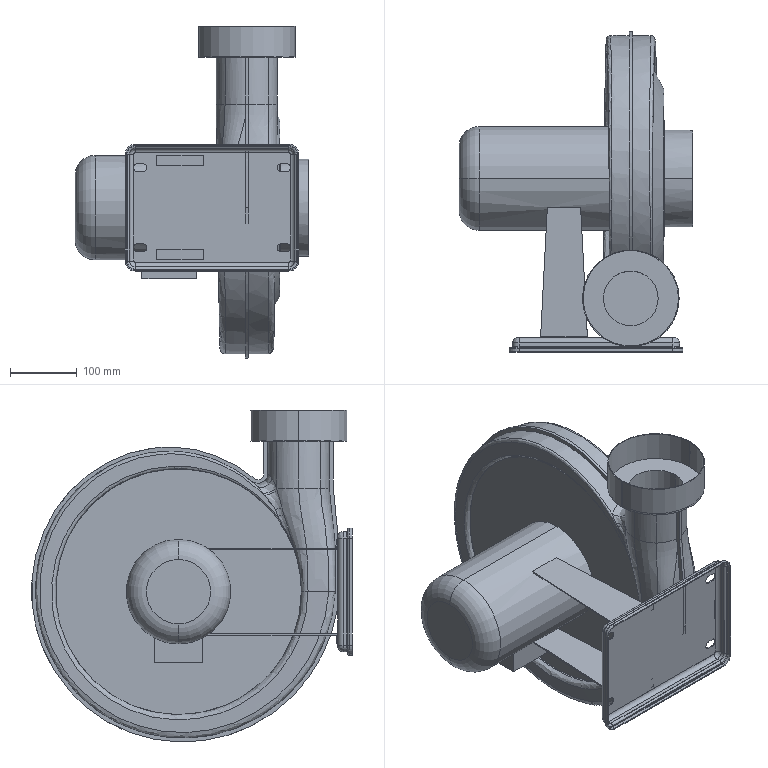Part | STEP file | 000 | 2 solids | 1638 faces | box 350 x 480.004 x 497.102 mm | volume 15476726 mm3 | plane 1483 | cylinder 65 | spline 51 | torus 28 | cone 8 | other 3 | commonest cylinder face diameters 4 x8 12 x8 30 x5 1 x4 7 x4 13 x4